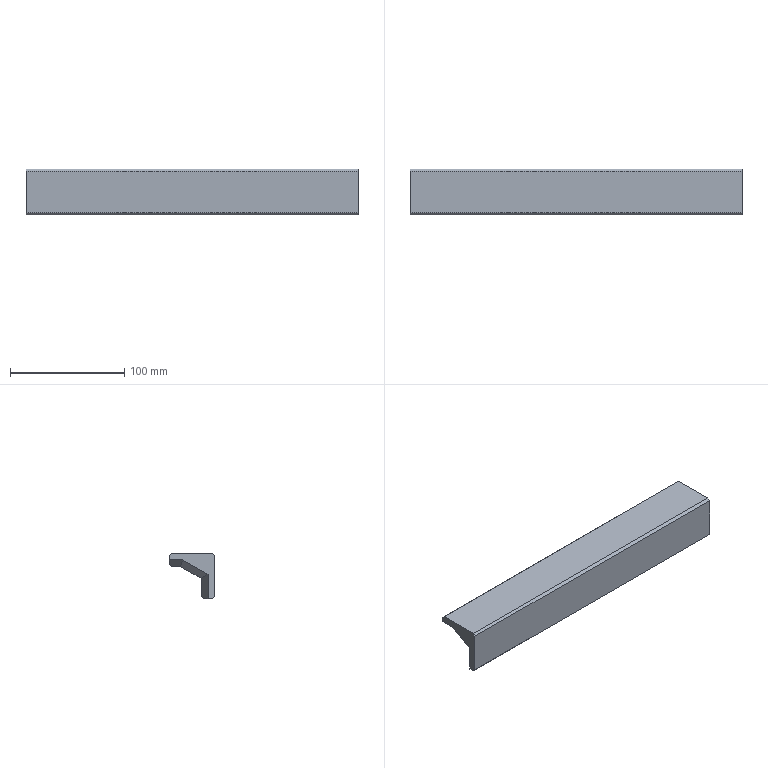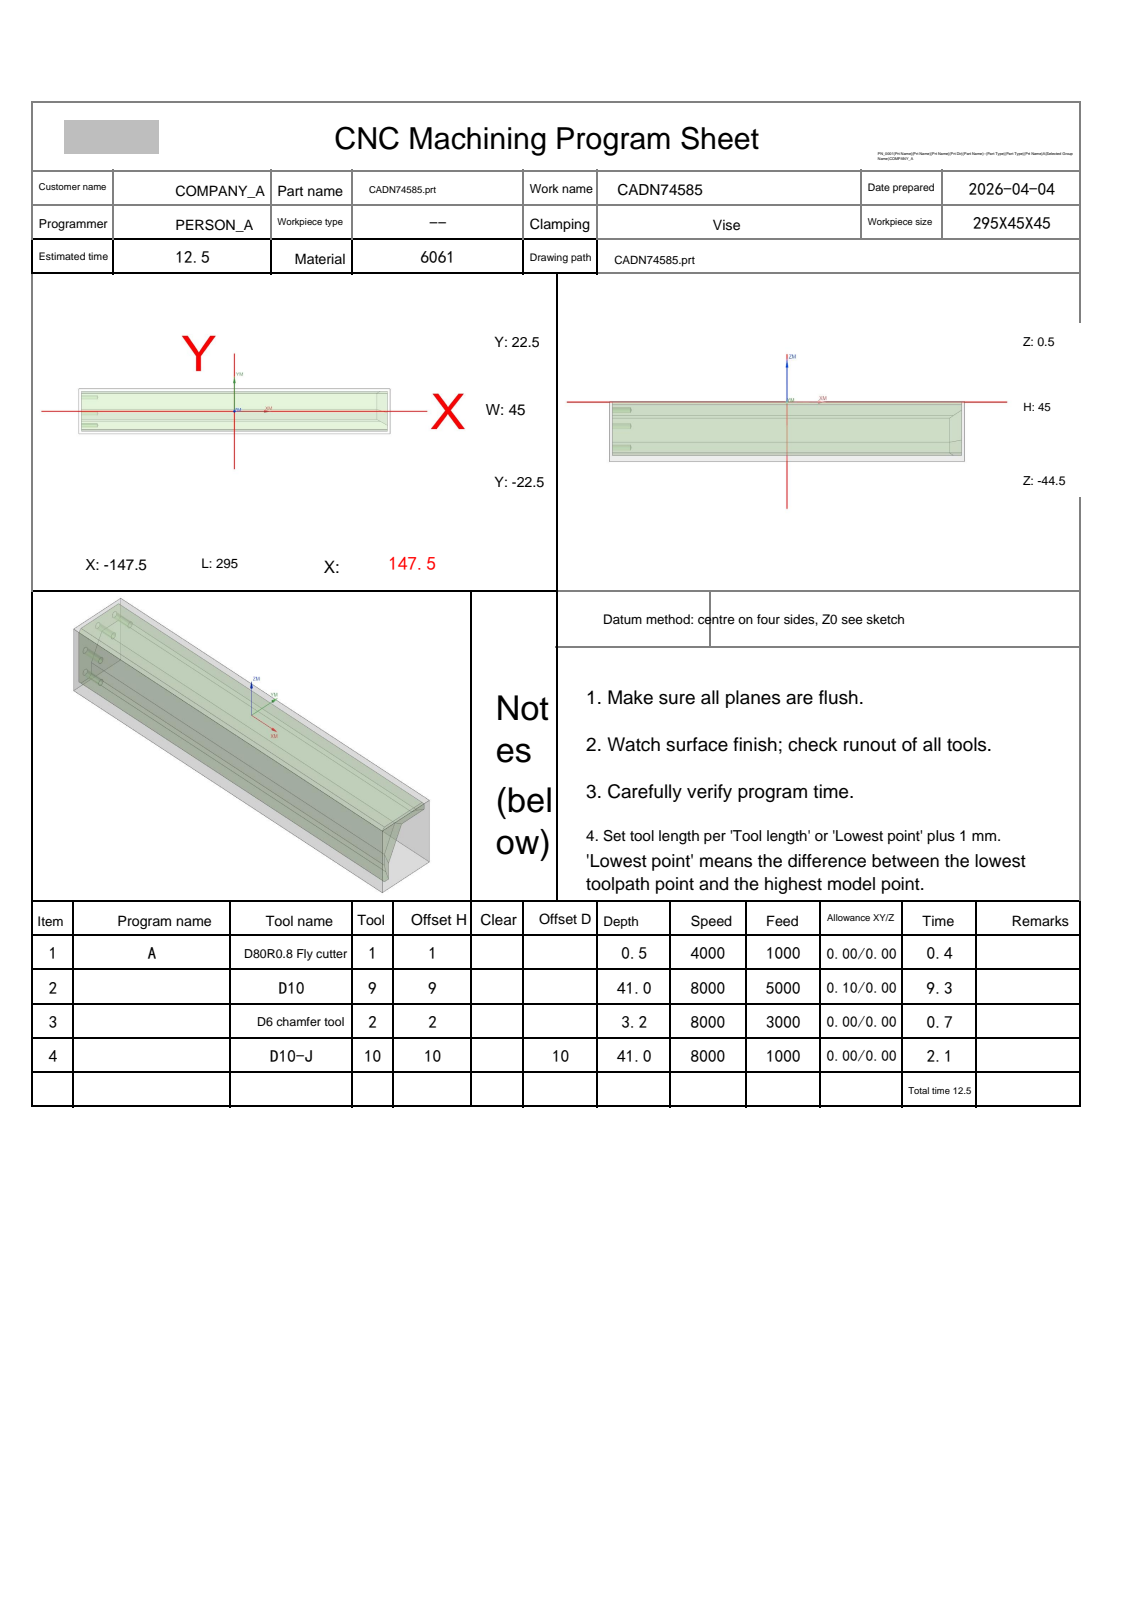NC program | NX | posted by the shop | part box 290 x 40 x 40 mm
Whole program:
%
O0001
(Machine time: 13.32 MIN)
(===Total Tool:4===)
(T1=D80R0.8 FlyCutter D=80.  R=0.8  D-  H01 Z=0.    )
(T9=D10     D=10.  R=0.   D-  H09 Z=-40.5 )
(T2=D6Chamfer   D=6.   R=0.   D-  H02 Z=-2.7  )
(T10=D10-J  D=10.  R=0.   D10 H10 Z=-40.5 )
G80 G90 G17 G49 G40
G91 G28 Z0
M01
N1 T01 M06
(D80R0.8 FlyCutter D=80. R=0.8 H=01 ce=0.00 di=0.00)
G00 G90 G54 X-190. Y0.0 M03 S4000
G43 H01 Z20.
M08
Z2.
G01 Z0.0 F1000.
X-185.
X185.
X190.
Z2.
G00 Z20.
G91 G28 Z0.0
M05
M09
G91 G28 Z0.0
M01
N2 T09 M06
(D10  D=10. R=0. H=09 ce=0.10 di=0.00)
G00 G90 G54 X0.0 Y-25.1 M03 S8000
G43 H09 Z20.
M08
Z.5
G01 X-145. Z.335 F5000.
G02 X-150.1 Y-20. Z.326 I0.0 J5.1
G01 Y20. Z.28
G02 X-145. Y25.1 Z.271 I5.1 J0.0
G01 X145. Z-.059
G02 X150.1 Y20. Z-.069 I0.0 J-5.1
G01 Y-20. Z-.114
G02 X145. Y-25.1 Z-.123 I-5.1 J0.0
G01 X-145. Z-.454
G02 X-150.1 Y-20. Z-.463 I0.0 J5.1
G01 Y20. Z-.508
G02 X-145. Y25.1 Z-.517 I5.1 J0.0
G01 X145. Z-.848
G02 X150.1 Y20. Z-.857 I0.0 J-5.1
G01 Y-20. Z-.903
G02 X145. Y-25.1 Z-.912 I-5.1 J0.0
G01 X-145. Z-1.242
G02 X-150.1 Y-20. Z-1.251 I0.0 J5.1
G01 Y20. Z-1.297
G02 X-145. Y25.1 Z-1.306 I5.1 J0.0
G01 X145. Z-1.636
G02 X150.1 Y20. Z-1.645 I0.0 J-5.1
G01 Y-20. Z-1.691
G02 X145. Y-25.1 Z-1.7 I-5.1 J0.0
G01 X-145. Z-2.031
G02 X-150.1 Y-20. Z-2.04 I0.0 J5.1
G01 Y20. Z-2.085
G02 X-145. Y25.1 Z-2.094 I5.1 J0.0
G01 X145. Z-2.425
G02 X150.1 Y20. Z-2.434 I0.0 J-5.1
G01 Y-20. Z-2.48
G02 X145. Y-25.1 Z-2.489 I-5.1 J0.0
G01 X-145. Z-2.819
G02 X-150.1 Y-20. Z-2.828 I0.0 J5.1
G01 Y20. Z-2.874
G02 X-145. Y25.1 Z-2.883 I5.1 J0.0
G01 X145. Z-3.213
G02 X150.1 Y20. Z-3.222 I0.0 J-5.1
G01 Y-20. Z-3.268
G02 X145. Y-25.1 Z-3.277 I-5.1 J0.0
G01 X-145. Z-3.608
G02 X-150.1 Y-20. Z-3.617 I0.0 J5.1
G01 Y20. Z-3.662
G02 X-145. Y25.1 Z-3.671 I5.1 J0.0
G01 X145. Z-4.002
G02 X150.1 Y20. Z-4.011 I0.0 J-5.1
G01 Y-20. Z-4.056
G02 X145. Y-25.1 Z-4.066 I-5.1 J0.0
G01 X-145. Z-4.396
G02 X-150.1 Y-20. Z-4.405 I0.0 J5.1
G01 Y20. Z-4.451
G02 X-145. Y25.1 Z-4.46 I5.1 J0.0
G01 X145. Z-4.79
G02 X150.1 Y20. Z-4.799 I0.0 J-5.1
G01 Y-20. Z-4.845
G02 X145. Y-25.1 Z-4.854 I-5.1 J0.0
G01 X-145. Z-5.184
G02 X-150.1 Y-20. Z-5.194 I0.0 J5.1
G01 Y20. Z-5.239
G02 X-145. Y25.1 Z-5.248 I5.1 J0.0
G01 X145. Z-5.579
G02 X150.1 Y20. Z-5.588 I0.0 J-5.1
G01 Y-20. Z-5.633
G02 X145. Y-25.1 Z-5.642 I-5.1 J0.0
G01 X-145. Z-5.973
G02 X-150.1 Y-20. Z-5.982 I0.0 J5.1
G01 Y20. Z-6.028
G02 X-145. Y25.1 Z-6.037 I5.1 J0.0
G01 X145. Z-6.367
G02 X150.1 Y20. Z-6.376 I0.0 J-5.1
G01 Y-20. Z-6.422
G02 X145. Y-25.1 Z-6.431 I-5.1 J0.0
G01 X-145. Z-6.761
G02 X-150.1 Y-20. Z-6.77 I0.0 J5.1
G01 Y20. Z-6.816
G02 X-145. Y25.1 Z-6.825 I5.1 J0.0
G01 X145. Z-7.156
G02 X150.1 Y20. Z-7.165 I0.0 J-5.1
G01 Y-20. Z-7.21
G02 X145. Y-25.1 Z-7.219 I-5.1 J0.0
G01 X-145. Z-7.55
G02 X-150.1 Y-20. Z-7.559 I0.0 J5.1
G01 Y20. Z-7.605
G02 X-145. Y25.1 Z-7.614 I5.1 J0.0
G01 X145. Z-7.944
G02 X150.1 Y20. Z-7.953 I0.0 J-5.1
G01 Y-20. Z-7.999
G02 X145. Y-25.1 Z-8.008 I-5.1 J0.0
G01 X-145. Z-8.338
G02 X-150.1 Y-20. Z-8.347 I0.0 J5.1
G01 Y20. Z-8.393
G02 X-145. Y25.1 Z-8.402 I5.1 J0.0
G01 X145. Z-8.733
G02 X150.1 Y20. Z-8.742 I0.0 J-5.1
G01 Y-20. Z-8.787
G02 X145. Y-25.1 Z-8.796 I-5.1 J0.0
G01 X-145. Z-9.127
G02 X-150.1 Y-20. Z-9.136 I0.0 J5.1
G01 Y20. Z-9.181
G02 X-145. Y25.1 Z-9.191 I5.1 J0.0
G01 X145. Z-9.521
G02 X150.1 Y20. Z-9.53 I0.0 J-5.1
G01 Y-20. Z-9.576
G02 X145. Y-25.1 Z-9.585 I-5.1 J0.0
G01 X-145. Z-9.915
G02 X-150.1 Y-20. Z-9.924 I0.0 J5.1
G01 Y20. Z-9.97
G02 X-145. Y25.1 Z-9.979 I5.1 J0.0
G01 X145. Z-10.309
G02 X150.1 Y20. Z-10.319 I0.0 J-5.1
G01 Y-20. Z-10.364
G02 X145. Y-25.1 Z-10.373 I-5.1 J0.0
G01 X-145. Z-10.704
G02 X-150.1 Y-20. Z-10.713 I0.0 J5.1
G01 Y20. Z-10.758
G02 X-145. Y25.1 Z-10.767 I5.1 J0.0
G01 X145. Z-11.098
G02 X150.1 Y20. Z-11.107 I0.0 J-5.1
G01 Y-20. Z-11.153
G02 X145. Y-25.1 Z-11.162 I-5.1 J0.0
G01 X-145. Z-11.492
G02 X-150.1 Y-20. Z-11.501 I0.0 J5.1
G01 Y20. Z-11.547
G02 X-145. Y25.1 Z-11.556 I5.1 J0.0
G01 X145. Z-11.886
G02 X150.1 Y20. Z-11.895 I0.0 J-5.1
G01 Y-20. Z-11.941
G02 X145. Y-25.1 Z-11.95 I-5.1 J0.0
G01 X-145. Z-12.281
G02 X-150.1 Y-20. Z-12.29 I0.0 J5.1
G01 Y20. Z-12.335
G02 X-145. Y25.1 Z-12.344 I5.1 J0.0
G01 X145. Z-12.675
G02 X150.1 Y20. Z-12.684 I0.0 J-5.1
G01 Y-20. Z-12.73
G02 X145. Y-25.1 Z-12.739 I-5.1 J0.0
G01 X-145. Z-13.069
G02 X-150.1 Y-20. Z-13.078 I0.0 J5.1
G01 Y20. Z-13.124
G02 X-145. Y25.1 Z-13.133 I5.1 J0.0
G01 X145. Z-13.463
G02 X150.1 Y20. Z-13.472 I0.0 J-5.1
G01 Y-20. Z-13.518
G02 X145. Y-25.1 Z-13.527 I-5.1 J0.0
G01 X-145. Z-13.858
G02 X-150.1 Y-20. Z-13.867 I0.0 J5.1
G01 Y20. Z-13.912
G02 X-145. Y25.1 Z-13.921 I5.1 J0.0
G01 X145. Z-14.252
G02 X150.1 Y20. Z-14.261 I0.0 J-5.1
G01 Y-20. Z-14.306
G02 X145. Y-25.1 Z-14.316 I-5.1 J0.0
G01 X-145. Z-14.646
G02 X-150.1 Y-20. Z-14.655 I0.0 J5.1
G01 Y20. Z-14.701
G02 X-145. Y25.1 Z-14.71 I5.1 J0.0
G01 X145. Z-15.04
G02 X150.1 Y20. Z-15.049 I0.0 J-5.1
G01 Y-20. Z-15.095
G02 X145. Y-25.1 Z-15.104 I-5.1 J0.0
G01 X-145. Z-15.434
G02 X-150.1 Y-20. Z-15.444 I0.0 J5.1
G01 Y20. Z-15.489
G02 X-145. Y25.1 Z-15.498 I5.1 J0.0
G01 X145. Z-15.829
G02 X150.1 Y20. Z-15.838 I0.0 J-5.1
G01 Y-20. Z-15.883
G02 X145. Y-25.1 Z-15.892 I-5.1 J0.0
G01 X-145. Z-16.223
G02 X-150.1 Y-20. Z-16.232 I0.0 J5.1
G01 Y20. Z-16.278
G02 X-145. Y25.1 Z-16.287 I5.1 J0.0
G01 X145. Z-16.617
G02 X150.1 Y20. Z-16.626 I0.0 J-5.1
G01 Y-20. Z-16.672
G02 X145. Y-25.1 Z-16.681 I-5.1 J0.0
G01 X-145. Z-17.011
G02 X-150.1 Y-20. Z-17.02 I0.0 J5.1
G01 Y20. Z-17.066
G02 X-145. Y25.1 Z-17.075 I5.1 J0.0
G01 X145. Z-17.406
G02 X150.1 Y20. Z-17.415 I0.0 J-5.1
G01 Y-20. Z-17.46
G02 X145. Y-25.1 Z-17.469 I-5.1 J0.0
G01 X-145. Z-17.8
G02 X-150.1 Y-20. Z-17.809 I0.0 J5.1
G01 Y20. Z-17.855
G02 X-145. Y25.1 Z-17.864 I5.1 J0.0
G01 X145. Z-18.194
G02 X150.1 Y20. Z-18.203 I0.0 J-5.1
G01 Y-20. Z-18.249
G02 X145. Y-25.1 Z-18.258 I-5.1 J0.0
G01 X-145. Z-18.588
G02 X-150.1 Y-20. Z-18.597 I0.0 J5.1
G01 Y20. Z-18.643
G02 X-145. Y25.1 Z-18.652 I5.1 J0.0
G01 X145. Z-18.983
G02 X150.1 Y20. Z-18.992 I0.0 J-5.1
G01 Y-20. Z-19.037
G02 X145. Y-25.1 Z-19.046 I-5.1 J0.0
G01 X-145. Z-19.377
G02 X-150.1 Y-20. Z-19.386 I0.0 J5.1
G01 Y20. Z-19.431
G02 X-145. Y25.1 Z-19.441 I5.1 J0.0
G01 X145. Z-19.771
G02 X150.1 Y20. Z-19.78 I0.0 J-5.1
G01 Y-20. Z-19.826
G02 X145. Y-25.1 Z-19.835 I-5.1 J0.0
G01 X-145. Z-20.165
G02 X-150.1 Y-20. Z-20.174 I0.0 J5.1
G01 Y20. Z-20.22
G02 X-145. Y25.1 Z-20.229 I5.1 J0.0
G01 X145. Z-20.559
G02 X150.1 Y20. Z-20.569 I0.0 J-5.1
G01 Y-20. Z-20.614
G02 X145. Y-25.1 Z-20.623 I-5.1 J0.0
G01 X-145. Z-20.954
G02 X-150.1 Y-20. Z-20.963 I0.0 J5.1
G01 Y20. Z-21.008
G02 X-145. Y25.1 Z-21.017 I5.1 J0.0
G01 X145. Z-21.348
G02 X150.1 Y20. Z-21.357 I0.0 J-5.1
G01 Y-20. Z-21.403
G02 X145. Y-25.1 Z-21.412 I-5.1 J0.0
G01 X-145. Z-21.742
G02 X-150.1 Y-20. Z-21.751 I0.0 J5.1
G01 Y20. Z-21.797
G02 X-145. Y25.1 Z-21.806 I5.1 J0.0
G01 X145. Z-22.136
G02 X150.1 Y20. Z-22.145 I0.0 J-5.1
G01 Y-20. Z-22.191
G02 X145. Y-25.1 Z-22.2 I-5.1 J0.0
G01 X-145. Z-22.531
G02 X-150.1 Y-20. Z-22.54 I0.0 J5.1
G01 Y20. Z-22.585
G02 X-145. Y25.1 Z-22.594 I5.1 J0.0
G01 X145. Z-22.925
G02 X150.1 Y20. Z-22.934 I0.0 J-5.1
G01 Y-20. Z-22.98
G02 X145. Y-25.1 Z-22.989 I-5.1 J0.0
G01 X-145. Z-23.319
G02 X-150.1 Y-20. Z-23.328 I0.0 J5.1
G01 Y20. Z-23.374
G02 X-145. Y25.1 Z-23.383 I5.1 J0.0
G01 X145. Z-23.713
G02 X150.1 Y20. Z-23.722 I0.0 J-5.1
G01 Y-20. Z-23.768
G02 X145. Y-25.1 Z-23.777 I-5.1 J0.0
G01 X-145. Z-24.108
G02 X-150.1 Y-20. Z-24.117 I0.0 J5.1
G01 Y20. Z-24.162
G02 X-145. Y25.1 Z-24.171 I5.1 J0.0
G01 X145. Z-24.502
G02 X150.1 Y20. Z-24.511 I0.0 J-5.1
G01 Y-20. Z-24.556
G02 X145. Y-25.1 Z-24.566 I-5.1 J0.0
G01 X-145. Z-24.896
G02 X-150.1 Y-20. Z-24.905 I0.0 J5.1
G01 Y20. Z-24.951
G02 X-145. Y25.1 Z-24.96 I5.1 J0.0
G01 X145. Z-25.29
G02 X150.1 Y20. Z-25.299 I0.0 J-5.1
G01 Y-20. Z-25.345
G02 X145. Y-25.1 Z-25.354 I-5.1 J0.0
G01 X-145. Z-25.684
G02 X-150.1 Y-20. Z-25.694 I0.0 J5.1
G01 Y20. Z-25.739
G02 X-145. Y25.1 Z-25.748 I5.1 J0.0
G01 X145. Z-26.079
G02 X150.1 Y20. Z-26.088 I0.0 J-5.1
G01 Y-20. Z-26.133
G02 X145. Y-25.1 Z-26.142 I-5.1 J0.0
G01 X-145. Z-26.473
G02 X-150.1 Y-20. Z-26.482 I0.0 J5.1
G01 Y20. Z-26.528
G02 X-145. Y25.1 Z-26.537 I5.1 J0.0
G01 X145. Z-26.867
G02 X150.1 Y20. Z-26.876 I0.0 J-5.1
G01 Y-20. Z-26.922
G02 X145. Y-25.1 Z-26.931 I-5.1 J0.0
G01 X-145. Z-27.261
G02 X-150.1 Y-20. Z-27.27 I0.0 J5.1
G01 Y20. Z-27.316
G02 X-145. Y25.1 Z-27.325 I5.1 J0.0
G01 X145. Z-27.656
G02 X150.1 Y20. Z-27.665 I0.0 J-5.1
G01 Y-20. Z-27.71
G02 X145. Y-25.1 Z-27.719 I-5.1 J0.0
G01 X-145. Z-28.05
G02 X-150.1 Y-20. Z-28.059 I0.0 J5.1
G01 Y20. Z-28.105
G02 X-145. Y25.1 Z-28.114 I5.1 J0.0
G01 X145. Z-28.444
G02 X150.1 Y20. Z-28.453 I0.0 J-5.1
G01 Y-20. Z-28.499
G02 X145. Y-25.1 Z-28.508 I-5.1 J0.0
G01 X-145. Z-28.838
G02 X-150.1 Y-20. Z-28.847 I0.0 J5.1
G01 Y20. Z-28.893
G02 X-145. Y25.1 Z-28.902 I5.1 J0.0
G01 X145. Z-29.233
G02 X150.1 Y20. Z-29.242 I0.0 J-5.1
G01 Y-20. Z-29.287
G02 X145. Y-25.1 Z-29.296 I-5.1 J0.0
G01 X-145. Z-29.627
G02 X-150.1 Y-20. Z-29.636 I0.0 J5.1
G01 Y20. Z-29.681
G02 X-145. Y25.1 Z-29.691 I5.1 J0.0
G01 X145. Z-30.021
G02 X150.1 Y20. Z-30.03 I0.0 J-5.1
G01 Y-20. Z-30.076
G02 X145. Y-25.1 Z-30.085 I-5.1 J0.0
G01 X-145. Z-30.415
G02 X-150.1 Y-20. Z-30.424 I0.0 J5.1
G01 Y20. Z-30.47
G02 X-145. Y25.1 Z-30.479 I5.1 J0.0
G01 X145. Z-30.809
G02 X150.1 Y20. Z-30.819 I0.0 J-5.1
G01 Y-20. Z-30.864
G02 X145. Y-25.1 Z-30.873 I-5.1 J0.0
G01 X-145. Z-31.204
G02 X-150.1 Y-20. Z-31.213 I0.0 J5.1
G01 Y20. Z-31.258
G02 X-145. Y25.1 Z-31.267 I5.1 J0.0
G01 X145. Z-31.598
G02 X150.1 Y20. Z-31.607 I0.0 J-5.1
G01 Y-20. Z-31.653
G02 X145. Y-25.1 Z-31.662 I-5.1 J0.0
G01 X-145. Z-31.992
G02 X-150.1 Y-20. Z-32.001 I0.0 J5.1
G01 Y20. Z-32.047
G02 X-145. Y25.1 Z-32.056 I5.1 J0.0
G01 X145. Z-32.386
G02 X150.1 Y20. Z-32.395 I0.0 J-5.1
G01 Y-20. Z-32.441
G02 X145. Y-25.1 Z-32.45 I-5.1 J0.0
G01 X-145. Z-32.781
G02 X-150.1 Y-20. Z-32.79 I0.0 J5.1
G01 Y20. Z-32.835
G02 X-145. Y25.1 Z-32.844 I5.1 J0.0
G01 X145. Z-33.175
G02 X150.1 Y20. Z-33.184 I0.0 J-5.1
G01 Y-20. Z-33.23
G02 X145. Y-25.1 Z-33.239 I-5.1 J0.0
G01 X-145. Z-33.569
G02 X-150.1 Y-20. Z-33.578 I0.0 J5.1
G01 Y20. Z-33.624
G02 X-145. Y25.1 Z-33.633 I5.1 J0.0
G01 X145. Z-33.963
G02 X150.1 Y20. Z-33.972 I0.0 J-5.1
G01 Y-20. Z-34.018
G02 X145. Y-25.1 Z-34.027 I-5.1 J0.0
G01 X-145. Z-34.358
G02 X-150.1 Y-20. Z-34.367 I0.0 J5.1
G01 Y20. Z-34.412
G02 X-145. Y25.1 Z-34.421 I5.1 J0.0
G01 X145. Z-34.752
G02 X150.1 Y20. Z-34.761 I0.0 J-5.1
G01 Y-20. Z-34.806
G02 X145. Y-25.1 Z-34.816 I-5.1 J0.0
G01 X-145. Z-35.146
G02 X-150.1 Y-20. Z-35.155 I0.0 J5.1
G01 Y20. Z-35.201
G02 X-145. Y25.1 Z-35.21 I5.1 J0.0
G01 X145. Z-35.54
G02 X150.1 Y20. Z-35.549 I0.0 J-5.1
G01 Y-20. Z-35.595
G02 X145. Y-25.1 Z-35.604 I-5.1 J0.0
G01 X-145. Z-35.934
G02 X-150.1 Y-20. Z-35.944 I0.0 J5.1
G01 Y20. Z-35.989
G02 X-145. Y25.1 Z-35.998 I5.1 J0.0
G01 X145. Z-36.329
G02 X150.1 Y20. Z-36.338 I0.0 J-5.1
G01 Y-20. Z-36.383
G02 X145. Y-25.1 Z-36.392 I-5.1 J0.0
G01 X-145. Z-36.723
G02 X-150.1 Y-20. Z-36.732 I0.0 J5.1
G01 Y20. Z-36.778
G02 X-145. Y25.1 Z-36.787 I5.1 J0.0
G01 X145. Z-37.117
G02 X150.1 Y20. Z-37.126 I0.0 J-5.1
G01 Y-20. Z-37.172
G02 X145. Y-25.1 Z-37.181 I-5.1 J0.0
G01 X-145. Z-37.511
G02 X-150.1 Y-20. Z-37.52 I0.0 J5.1
G01 Y20. Z-37.566
G02 X-145. Y25.1 Z-37.575 I5.1 J0.0
G01 X145. Z-37.906
G02 X150.1 Y20. Z-37.915 I0.0 J-5.1
G01 Y-20. Z-37.96
G02 X145. Y-25.1 Z-37.969 I-5.1 J0.0
G01 X-145. Z-38.3
G02 X-150.1 Y-20. Z-38.309 I0.0 J5.1
G01 Y20. Z-38.355
G02 X-145. Y25.1 Z-38.364 I5.1 J0.0
G01 X145. Z-38.694
G02 X150.1 Y20. Z-38.703 I0.0 J-5.1
G01 Y-20. Z-38.749
G02 X145. Y-25.1 Z-38.758 I-5.1 J0.0
G01 X-145. Z-39.088
G02 X-150.1 Y-20. Z-39.097 I0.0 J5.1
G01 Y20. Z-39.143
G02 X-145. Y25.1 Z-39.152 I5.1 J0.0
G01 X145. Z-39.483
G02 X150.1 Y20. Z-39.492 I0.0 J-5.1
G01 Y-20. Z-39.537
G02 X145. Y-25.1 Z-39.546 I-5.1 J0.0
G01 X-145. Z-39.877
G02 X-150.1 Y-20. Z-39.886 I0.0 J5.1
G01 Y20. Z-39.931
G02 X-145. Y25.1 Z-39.941 I5.1 J0.0
G01 X145. Z-40.271
G02 X150.1 Y20. Z-40.28 I0.0 J-5.1
G01 Y-20. Z-40.326
G02 X145. Y-25.1 Z-40.335 I-5.1 J0.0
G01 X0.0 Z-40.5
X-145.
G02 X-150.1 Y-20. I0.0 J5.1
G01 Y20.
G02 X-145. Y25.1 I5.1 J0.0
G01 X145.
G02 X150.1 Y20. I0.0 J-5.1
G01 Y-20.
G02 X145. Y-25.1 I-5.1 J0.0
G01 X0.0
X-.5
Z-39.5
G00 Z20.
G00 G90 X-154.936 Y22.983 M03 S7000
Z10.878
Z.359
G01 Z-.141 F4500.
X-146.072 Y23.239
X-145.985 Y23.241
X145.985
X146.072 Y23.239
Y23.312 Z-.212
Y23.38 Z-.283
X145.985 Y23.383
X-145.985
X-146.072 Y23.38
Y23.454 Z-.354
Y23.522 Z-.424
X-145.985 Y23.524
X145.985
X146.072 Y23.522
Y23.595 Z-.495
X146.073 Y23.663 Z-.566
X145.985 Y23.666
X-145.985
X-146.073 Y23.663
Y23.736 Z-.636
Y23.805 Z-.707
X-145.985 Y23.807
X145.985
X146.073 Y23.805
Y23.878 Z-.778
Y23.946 Z-.849
X145.985 Y23.949
X-145.985
X-146.073 Y23.946
Y24.019 Z-.919
Y24.087 Z-.99
X-145.985 Y24.09
X145.985
X146.073 Y24.087
Y24.161 Z-1.061
Y24.229 Z-1.131
X145.985 Y24.231
X-145.985
X-146.073 Y24.229
Y24.302 Z-1.202
Y24.37 Z-1.273
X-145.985 Y24.373
X145.985
X146.073 Y24.37
Y24.444 Z-1.344
Y24.512 Z-1.414
X145.985 Y24.514
X-145.985
X-146.073 Y24.512
X-146.072 Y24.585 Z-1.485
Y24.653 Z-1.556
X-145.985 Y24.656
X145.985
X146.072 Y24.653
Y24.711 Z-1.611
Y24.764 Z-1.667
X145.985 Y24.767
X-145.985
X-146.072 Y24.764
Y24.822 Z-1.722
Y24.875 Z-1.778
X-145.985 Y24.878
X145.985
X146.072 Y24.875
Y24.933 Z-1.833
Y24.986 Z-1.889
X145.985 Y24.989
X-145.985
X-146.072 Y24.986
Y25.044 Z-1.944
Y25.097 Z-2.
X146.072
G00 Z10.878
X154.936 Y-22.983
Z.359
G01 Z-.141
X146.072 Y-23.239
X145.985 Y-23.241
X-145.985
X-146.072 Y-23.239
Y-23.312 Z-.212
Y-23.38 Z-.283
X-145.985 Y-23.383
X145.985
X146.072 Y-23.38
Y-23.454 Z-.354
Y-23.522 Z-.424
X145.985 Y-23.524
X-145.985
X-146.072 Y-23.522
Y-23.595 Z-.495
X-146.073 Y-23.663 Z-.566
X-145.985 Y-23.666
X145.985
X146.073 Y-23.663
Y-23.736 Z-.636
Y-23.805 Z-.707
X145.985 Y-23.807
X-145.985
X-146.073 Y-23.805
Y-23.878 Z-.778
Y-23.946 Z-.849
X-145.985 Y-23.949
X145.985
X146.073 Y-23.946
Y-24.019 Z-.919
Y-24.087 Z-.99
X145.985 Y-24.09
X-145.985
X-146.073 Y-24.087
Y-24.161 Z-1.061
Y-24.229 Z-1.131
X-145.985 Y-24.231
X145.985
X146.073 Y-24.229
Y-24.302 Z-1.202
Y-24.37 Z-1.273
X145.985 Y-24.373
X-145.985
X-146.073 Y-24.37
Y-24.444 Z-1.344
Y-24.512 Z-1.414
X-145.985 Y-24.514
X145.985
X146.073 Y-24.512
X146.072 Y-24.585 Z-1.485
Y-24.653 Z-1.556
X145.985 Y-24.656
X-145.985
X-146.072 Y-24.653
Y-24.711 Z-1.611
Y-24.764 Z-1.667
X-145.985 Y-24.767
X145.985
X146.072 Y-24.764
Y-24.822 Z-1.722
Y-24.875 Z-1.778
X145.985 Y-24.878
X-145.985
X-146.072 Y-24.875
Y-24.933 Z-1.833
Y-24.986 Z-1.889
X-145.985 Y-24.989
X145.985
X146.072 Y-24.986
Y-25.044 Z-1.944
Y-25.097 Z-2.
X-146.072
G00 Z10.878
G91 G28 Z0.0
M05
M09
G91 G28 Z0.0
M01
N3 T02 M06
(D6Chamfer D=6. R=0. H=02 ce=0.00 di=0.00)
G00 G90 G54 X-148.9 Y21.516 M03 S6500
G43 H02 Z20.
M08
Z-1.2
G01 Z-2.7 F1000.
G03 X-147.763 Y20.7 I1.137 J.384
G01 X147.763
G03 X148.9 Y21.516 I0.0 J1.2
G01 Z-1.2
G00 Z20.
Y-21.516
Z-1.2
G01 Z-2.7
G03 X147.763 Y-20.7 I-1.137 J-.384
G01 X-147.763
G03 X-148.9 Y-21.516 I0.0 J-1.2
G01 Z-1.2
G00 Z20.
G00 G90 X-146.207 Y-18.461 M03 S8000
Z20.
Z2.935
G01 Z-1.5 F3000.
X-146.267 Y-18.289
X-146.3 Y-18.
Y18.
X-146.267 Y18.289
X-146.207 Y18.461
Z2.935
G00 Z20.
X146.207
Z2.935
G01 Z-1.5
X146.267 Y18.289
X146.3 Y18.
Y-18.
X146.267 Y-18.289
X146.207 Y-18.461
Z2.935
G00 Z20.
G91 G28 Z0.0
M05
M09
G91 G28 Z0.0
M01
N4 T10 M06
(D10-J  D=10. R=0. H=10 ce=0.00 di=0.00)
G00 G90 G54 X-146.013 Y26.116 M03 S8000
G43 H10 Z20.
M08
Z-13.
G01 Z-13.5 F1000.
G41 D10
X-145.997 Y25.917
G03 X-145. Y25. I.997 J.083
G01 X145.
G02 X150. Y20. I0.0 J-5.
G01 Y-20.
G02 X145. Y-25. I-5. J0.0
G01 X-145.
G02 X-150. Y-20. I0.0 J5.
G01 Y20.
G02 X-145. Y25. I5. J0.0
G01 X-144.5
G03 X-143.5 Y26. I0.0 J1.
G01 G40 Y26.2
Z-13.
G00 Z20.
X-146.013 Y26.116
Z-26.5
G01 Z-27.
G41 D10
X-145.997 Y25.917
G03 X-145. Y25. I.997 J.083
G01 X145.
G02 X150. Y20. I0.0 J-5.
G01 Y-20.
G02 X145. Y-25. I-5. J0.0
G01 X-145.
G02 X-150. Y-20. I0.0 J5.
G01 Y20.
G02 X-145. Y25. I5. J0.0
G01 X-144.5
G03 X-143.5 Y26. I0.0 J1.
G01 G40 Y26.2
Z-26.5
G00 Z20.
X-146.013 Y26.116
Z-40.
G01 Z-40.5
G41 D10
X-145.997 Y25.917
G03 X-145. Y25. I.997 J.083
G01 X145.
G02 X150. Y20. I0.0 J-5.
G01 Y-20.
G02 X145. Y-25. I-5. J0.0
G01 X-145.
G02 X-150. Y-20. I0.0 J5.
G01 Y20.
G02 X-145. Y25. I5. J0.0
G01 X-144.5
G03 X-143.5 Y26. I0.0 J1.
G01 G40 Y26.2
Z-40.
G00 Z20.
M05
M09
G91 G28 Z0.0
G91 G28 Y0.0
M30
%